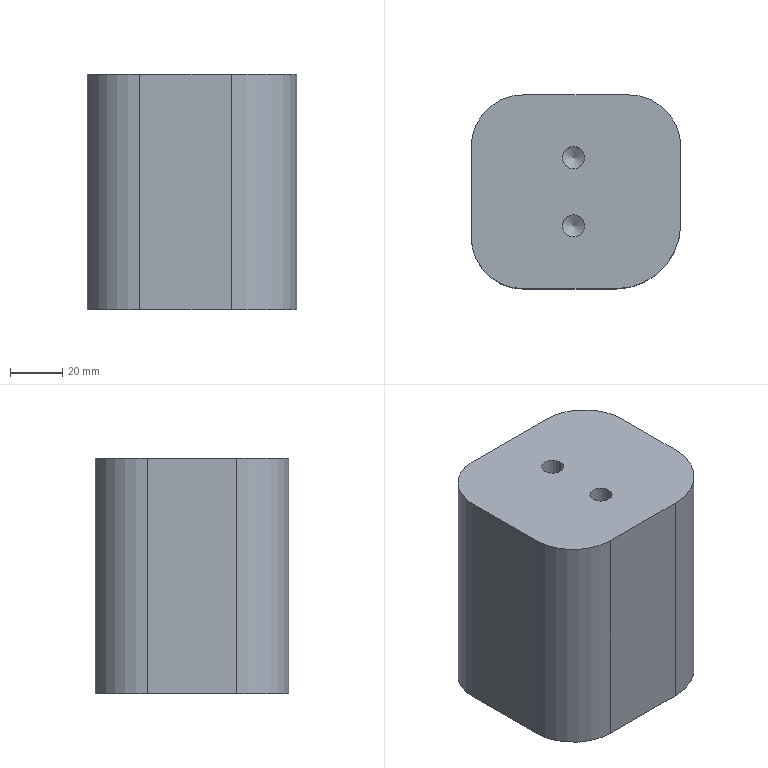Part | STEP file | gslz 2016.10.28-10_id2266_x_t | 1 solid | 58 faces | box 80 x 74 x 90 mm | volume 484715 mm3 | spline 41 | plane 7 | cylinder 6 | sphere 2 | cone 2 | commonest cylinder face diameters 40 x3 8.5 x2 50 x1